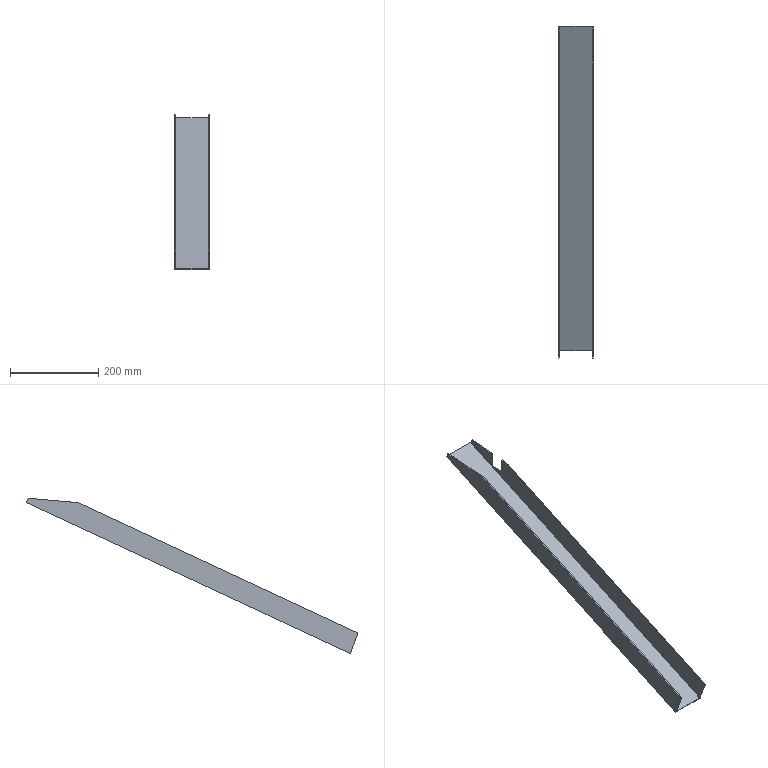Part | NX | features solid 2 | 1 solid | 16 faces | box 78 x 752.166 x 352.381 mm | volume 271303 mm3 | plane 16
STEP:
#1=CARTESIAN_POINT('',(843.,225.865,-160.385));
#2=VERTEX_POINT('',#1);
#3=CARTESIAN_POINT('',(843.,245.,-158.711));
#4=VERTEX_POINT('',#3);
#5=CARTESIAN_POINT('',(843.,-931.001,-261.597));
#6=DIRECTION('',(0.,0.9962,0.08716));
#7=VECTOR('',#6,1000.);
#8=LINE('',#5,#7);
#9=EDGE_CURVE('',#2,#4,#8,.T.);
#10=ORIENTED_EDGE('',*,*,#9,.T.);
#11=CARTESIAN_POINT('',(843.,245.,-190.));
#12=VERTEX_POINT('',#11);
#13=CARTESIAN_POINT('',(843.,245.,-735.668));
#14=DIRECTION('',(0.,0.,-1.));
#15=VECTOR('',#14,1000.);
#16=LINE('',#13,#15);
#17=EDGE_CURVE('',#4,#12,#16,.T.);
#18=ORIENTED_EDGE('',*,*,#17,.T.);
#19=CARTESIAN_POINT('',(843.,275.,-190.));
#20=VERTEX_POINT('',#19);
#21=CARTESIAN_POINT('',(843.,-889.525,-190.));
#22=DIRECTION('',(0.,1.,0.));
#23=VECTOR('',#22,1000.);
#24=LINE('',#21,#23);
#25=EDGE_CURVE('',#12,#20,#24,.T.);
#26=ORIENTED_EDGE('',*,*,#25,.T.);
#27=CARTESIAN_POINT('',(843.,275.,-156.086));
#28=VERTEX_POINT('',#27);
#29=CARTESIAN_POINT('',(843.,275.,-735.668));
#30=DIRECTION('',(0.,0.,-1.));
#31=VECTOR('',#30,1000.);
#32=LINE('',#29,#31);
#33=EDGE_CURVE('',#28,#20,#32,.T.);
#34=ORIENTED_EDGE('',*,*,#33,.F.);
#35=CARTESIAN_POINT('',(843.,340.503,-150.355));
#36=VERTEX_POINT('',#35);
#37=CARTESIAN_POINT('',(843.,-931.001,-261.597));
#38=DIRECTION('',(0.,0.9962,0.08716));
#39=VECTOR('',#38,1000.);
#40=LINE('',#37,#39);
#41=EDGE_CURVE('',#28,#36,#40,.T.);
#42=ORIENTED_EDGE('',*,*,#41,.T.);
#43=CARTESIAN_POINT('',(843.,344.155,-158.187));
#44=VERTEX_POINT('',#43);
#45=CARTESIAN_POINT('',(843.,345.,-160.));
#46=DIRECTION('',(0.,-0.4226,0.9063));
#47=VECTOR('',#46,1000.);
#48=LINE('',#45,#47);
#49=EDGE_CURVE('',#44,#36,#48,.T.);
#50=ORIENTED_EDGE('',*,*,#49,.F.);
#51=CARTESIAN_POINT('',(843.,-390.687,-500.85));
#52=VERTEX_POINT('',#51);
#53=CARTESIAN_POINT('',(843.,-71.454,-351.989));
#54=DIRECTION('',(0.,-0.9063,-0.4226));
#55=VECTOR('',#54,1000.);
#56=LINE('',#53,#55);
#57=EDGE_CURVE('',#44,#52,#56,.T.);
#58=ORIENTED_EDGE('',*,*,#57,.T.);
#59=CARTESIAN_POINT('',(843.,-407.166,-455.572));
#60=VERTEX_POINT('',#59);
#61=CARTESIAN_POINT('',(843.,-373.57,-547.876));
#62=DIRECTION('',(0.,-0.342,0.9397));
#63=VECTOR('',#62,1000.);
#64=LINE('',#61,#63);
#65=EDGE_CURVE('',#52,#60,#64,.T.);
#66=ORIENTED_EDGE('',*,*,#65,.T.);
#67=CARTESIAN_POINT('',(843.,-910.656,-690.353));
#68=DIRECTION('',(0.,-0.9063,-0.4226));
#69=VECTOR('',#68,1000.);
#70=LINE('',#67,#69);
#71=EDGE_CURVE('',#60,#2,#70,.F.);
#72=ORIENTED_EDGE('',*,*,#71,.T.);
#73=EDGE_LOOP('',(#10,#18,#26,#34,#42,#50,#58,#66,#72));
#74=FACE_BOUND('',#73,.T.);
#75=CARTESIAN_POINT('',(843.,-889.525,-735.668));
#76=DIRECTION('',(-1.,0.,0.));
#77=DIRECTION('',(0.,0.08716,-0.9962));
#78=AXIS2_PLACEMENT_3D('',#75,#76,#77);
#79=PLANE('',#78);
#80=ADVANCED_FACE('',(#74),#79,.T.);
#81=CARTESIAN_POINT('',(845.,275.,-190.));
#82=VERTEX_POINT('',#81);
#83=CARTESIAN_POINT('',(845.,245.,-190.));
#84=VERTEX_POINT('',#83);
#85=CARTESIAN_POINT('',(845.,-890.37,-190.));
#86=DIRECTION('',(0.,-1.,0.));
#87=VECTOR('',#86,1000.);
#88=LINE('',#85,#87);
#89=EDGE_CURVE('',#82,#84,#88,.T.);
#90=ORIENTED_EDGE('',*,*,#89,.T.);
#91=CARTESIAN_POINT('',(845.,245.,-158.711));
#92=VERTEX_POINT('',#91);
#93=CARTESIAN_POINT('',(845.,245.,-733.856));
#94=DIRECTION('',(0.,0.,1.));
#95=VECTOR('',#94,1000.);
#96=LINE('',#93,#95);
#97=EDGE_CURVE('',#84,#92,#96,.T.);
#98=ORIENTED_EDGE('',*,*,#97,.T.);
#99=CARTESIAN_POINT('',(845.,225.865,-160.385));
#100=VERTEX_POINT('',#99);
#101=CARTESIAN_POINT('',(845.,-931.682,-261.657));
#102=DIRECTION('',(0.,-0.9962,-0.08716));
#103=VECTOR('',#102,1000.);
#104=LINE('',#101,#103);
#105=EDGE_CURVE('',#92,#100,#104,.T.);
#106=ORIENTED_EDGE('',*,*,#105,.T.);
#107=CARTESIAN_POINT('',(845.,-407.166,-455.572));
#108=VERTEX_POINT('',#107);
#109=CARTESIAN_POINT('',(845.,-910.656,-690.353));
#110=DIRECTION('',(0.,-0.9063,-0.4226));
#111=VECTOR('',#110,1000.);
#112=LINE('',#109,#111);
#113=EDGE_CURVE('',#108,#100,#112,.F.);
#114=ORIENTED_EDGE('',*,*,#113,.F.);
#115=CARTESIAN_POINT('',(845.,-390.,-502.736));
#116=VERTEX_POINT('',#115);
#117=CARTESIAN_POINT('',(845.,-374.252,-546.004));
#118=DIRECTION('',(0.,0.342,-0.9397));
#119=VECTOR('',#118,1000.);
#120=LINE('',#117,#119);
#121=EDGE_CURVE('',#108,#116,#120,.T.);
#122=ORIENTED_EDGE('',*,*,#121,.T.);
#123=CARTESIAN_POINT('',(845.,345.,-160.));
#124=VERTEX_POINT('',#123);
#125=CARTESIAN_POINT('',(845.,-70.609,-353.802));
#126=DIRECTION('',(0.,0.9063,0.4226));
#127=VECTOR('',#126,1000.);
#128=LINE('',#125,#127);
#129=EDGE_CURVE('',#116,#124,#128,.T.);
#130=ORIENTED_EDGE('',*,*,#129,.T.);
#131=CARTESIAN_POINT('',(845.,340.503,-150.355));
#132=VERTEX_POINT('',#131);
#133=CARTESIAN_POINT('',(845.,344.155,-158.187));
#134=DIRECTION('',(0.,0.4226,-0.9063));
#135=VECTOR('',#134,1000.);
#136=LINE('',#133,#135);
#137=EDGE_CURVE('',#132,#124,#136,.T.);
#138=ORIENTED_EDGE('',*,*,#137,.F.);
#139=CARTESIAN_POINT('',(845.,275.,-156.086));
#140=VERTEX_POINT('',#139);
#141=CARTESIAN_POINT('',(845.,-931.682,-261.657));
#142=DIRECTION('',(0.,-0.9962,-0.08716));
#143=VECTOR('',#142,1000.);
#144=LINE('',#141,#143);
#145=EDGE_CURVE('',#132,#140,#144,.T.);
#146=ORIENTED_EDGE('',*,*,#145,.T.);
#147=CARTESIAN_POINT('',(845.,275.,-733.856));
#148=DIRECTION('',(0.,0.,1.));
#149=VECTOR('',#148,1000.);
#150=LINE('',#147,#149);
#151=EDGE_CURVE('',#82,#140,#150,.T.);
#152=ORIENTED_EDGE('',*,*,#151,.F.);
#153=EDGE_LOOP('',(#90,#98,#106,#114,#122,#130,#138,#146,#152));
#154=FACE_BOUND('',#153,.T.);
#155=CARTESIAN_POINT('',(845.,-890.37,-733.856));
#156=DIRECTION('',(1.,0.,0.));
#157=DIRECTION('',(0.,-0.08716,0.9962));
#158=AXIS2_PLACEMENT_3D('',#155,#156,#157);
#159=PLANE('',#158);
#160=ADVANCED_FACE('',(#154),#159,.T.);
#161=CARTESIAN_POINT('',(827.,245.,-158.711));
#162=DIRECTION('',(1.,0.,0.));
#163=VECTOR('',#162,1000.);
#164=LINE('',#161,#163);
#165=EDGE_CURVE('',#4,#92,#164,.T.);
#166=ORIENTED_EDGE('',*,*,#165,.F.);
#167=ORIENTED_EDGE('',*,*,#9,.F.);
#168=CARTESIAN_POINT('',(820.,225.865,-160.385));
#169=DIRECTION('',(1.,0.,0.));
#170=VECTOR('',#169,1000.);
#171=LINE('',#168,#170);
#172=EDGE_CURVE('',#100,#2,#171,.F.);
#173=ORIENTED_EDGE('',*,*,#172,.F.);
#174=ORIENTED_EDGE('',*,*,#105,.F.);
#175=EDGE_LOOP('',(#166,#167,#173,#174));
#176=FACE_BOUND('',#175,.T.);
#177=CARTESIAN_POINT('',(827.,314.243,-152.653));
#178=DIRECTION('',(0.,0.08716,-0.9962));
#179=DIRECTION('',(1.,0.,0.));
#180=AXIS2_PLACEMENT_3D('',#177,#178,#179);
#181=PLANE('',#180);
#182=ADVANCED_FACE('',(#176),#181,.F.);
#183=CARTESIAN_POINT('',(767.,-390.,-502.736));
#184=VERTEX_POINT('',#183);
#185=CARTESIAN_POINT('',(905.,-390.,-502.736));
#186=DIRECTION('',(-1.,0.,0.));
#187=VECTOR('',#186,1000.);
#188=LINE('',#185,#187);
#189=EDGE_CURVE('',#116,#184,#188,.T.);
#190=ORIENTED_EDGE('',*,*,#189,.T.);
#191=CARTESIAN_POINT('',(767.,345.,-160.));
#192=VERTEX_POINT('',#191);
#193=CARTESIAN_POINT('',(767.,-70.609,-353.802));
#194=DIRECTION('',(0.,0.9063,0.4226));
#195=VECTOR('',#194,1000.);
#196=LINE('',#193,#195);
#197=EDGE_CURVE('',#184,#192,#196,.T.);
#198=ORIENTED_EDGE('',*,*,#197,.T.);
#199=CARTESIAN_POINT('',(1300.,345.,-160.));
#200=DIRECTION('',(-1.,0.,0.));
#201=VECTOR('',#200,1000.);
#202=LINE('',#199,#201);
#203=EDGE_CURVE('',#124,#192,#202,.T.);
#204=ORIENTED_EDGE('',*,*,#203,.F.);
#205=ORIENTED_EDGE('',*,*,#129,.F.);
#206=EDGE_LOOP('',(#190,#198,#204,#205));
#207=FACE_BOUND('',#206,.T.);
#208=CARTESIAN_POINT('',(905.,-70.609,-353.802));
#209=DIRECTION('',(0.,0.4226,-0.9063));
#210=DIRECTION('',(0.,0.9063,0.4226));
#211=AXIS2_PLACEMENT_3D('',#208,#209,#210);
#212=PLANE('',#211);
#213=ADVANCED_FACE('',(#207),#212,.T.);
#214=CARTESIAN_POINT('',(769.,-407.166,-455.572));
#215=VERTEX_POINT('',#214);
#216=CARTESIAN_POINT('',(769.,225.865,-160.385));
#217=VERTEX_POINT('',#216);
#218=CARTESIAN_POINT('',(769.,-910.656,-690.353));
#219=DIRECTION('',(0.,0.9063,0.4226));
#220=VECTOR('',#219,1000.);
#221=LINE('',#218,#220);
#222=EDGE_CURVE('',#215,#217,#221,.T.);
#223=ORIENTED_EDGE('',*,*,#222,.T.);
#224=CARTESIAN_POINT('',(767.,225.865,-160.385));
#225=VERTEX_POINT('',#224);
#226=CARTESIAN_POINT('',(750.,225.865,-160.385));
#227=DIRECTION('',(1.,0.,0.));
#228=VECTOR('',#227,1000.);
#229=LINE('',#226,#228);
#230=EDGE_CURVE('',#225,#217,#229,.T.);
#231=ORIENTED_EDGE('',*,*,#230,.F.);
#232=CARTESIAN_POINT('',(767.,-407.166,-455.572));
#233=VERTEX_POINT('',#232);
#234=CARTESIAN_POINT('',(767.,-910.656,-690.353));
#235=DIRECTION('',(0.,0.9063,0.4226));
#236=VECTOR('',#235,1000.);
#237=LINE('',#234,#236);
#238=EDGE_CURVE('',#233,#225,#237,.T.);
#239=ORIENTED_EDGE('',*,*,#238,.F.);
#240=CARTESIAN_POINT('',(750.,-407.166,-455.572));
#241=DIRECTION('',(-1.,0.,0.));
#242=VECTOR('',#241,1000.);
#243=LINE('',#240,#242);
#244=EDGE_CURVE('',#215,#233,#243,.T.);
#245=ORIENTED_EDGE('',*,*,#244,.F.);
#246=EDGE_LOOP('',(#223,#231,#239,#245));
#247=FACE_BOUND('',#246,.T.);
#248=CARTESIAN_POINT('',(750.,-910.656,-690.353));
#249=DIRECTION('',(0.,0.4226,-0.9063));
#250=DIRECTION('',(0.,0.9063,0.4226));
#251=AXIS2_PLACEMENT_3D('',#248,#249,#250);
#252=PLANE('',#251);
#253=ADVANCED_FACE('',(#247),#252,.F.);
#254=CARTESIAN_POINT('',(769.,344.155,-158.187));
#255=VERTEX_POINT('',#254);
#256=CARTESIAN_POINT('',(769.,-390.687,-500.85));
#257=VERTEX_POINT('',#256);
#258=CARTESIAN_POINT('',(769.,-71.454,-351.989));
#259=DIRECTION('',(0.,-0.9063,-0.4226));
#260=VECTOR('',#259,1000.);
#261=LINE('',#258,#260);
#262=EDGE_CURVE('',#255,#257,#261,.T.);
#263=ORIENTED_EDGE('',*,*,#262,.F.);
#264=CARTESIAN_POINT('',(769.,340.503,-150.355));
#265=VERTEX_POINT('',#264);
#266=CARTESIAN_POINT('',(769.,345.,-160.));
#267=DIRECTION('',(0.,-0.4226,0.9063));
#268=VECTOR('',#267,1000.);
#269=LINE('',#266,#268);
#270=EDGE_CURVE('',#255,#265,#269,.T.);
#271=ORIENTED_EDGE('',*,*,#270,.T.);
#272=CARTESIAN_POINT('',(769.,-931.001,-261.597));
#273=DIRECTION('',(0.,0.9962,0.08716));
#274=VECTOR('',#273,1000.);
#275=LINE('',#272,#274);
#276=EDGE_CURVE('',#217,#265,#275,.T.);
#277=ORIENTED_EDGE('',*,*,#276,.F.);
#278=ORIENTED_EDGE('',*,*,#222,.F.);
#279=CARTESIAN_POINT('',(769.,-373.57,-547.876));
#280=DIRECTION('',(0.,-0.342,0.9397));
#281=VECTOR('',#280,1000.);
#282=LINE('',#279,#281);
#283=EDGE_CURVE('',#257,#215,#282,.T.);
#284=ORIENTED_EDGE('',*,*,#283,.F.);
#285=EDGE_LOOP('',(#263,#271,#277,#278,#284));
#286=FACE_BOUND('',#285,.T.);
#287=CARTESIAN_POINT('',(769.,-889.525,-735.668));
#288=DIRECTION('',(-1.,0.,0.));
#289=DIRECTION('',(0.,0.08716,-0.9962));
#290=AXIS2_PLACEMENT_3D('',#287,#288,#289);
#291=PLANE('',#290);
#292=ADVANCED_FACE('',(#286),#291,.F.);
#293=ORIENTED_EDGE('',*,*,#238,.T.);
#294=CARTESIAN_POINT('',(767.,340.503,-150.355));
#295=VERTEX_POINT('',#294);
#296=CARTESIAN_POINT('',(767.,-931.682,-261.657));
#297=DIRECTION('',(0.,-0.9962,-0.08716));
#298=VECTOR('',#297,1000.);
#299=LINE('',#296,#298);
#300=EDGE_CURVE('',#295,#225,#299,.T.);
#301=ORIENTED_EDGE('',*,*,#300,.F.);
#302=CARTESIAN_POINT('',(767.,344.155,-158.187));
#303=DIRECTION('',(0.,0.4226,-0.9063));
#304=VECTOR('',#303,1000.);
#305=LINE('',#302,#304);
#306=EDGE_CURVE('',#295,#192,#305,.T.);
#307=ORIENTED_EDGE('',*,*,#306,.T.);
#308=ORIENTED_EDGE('',*,*,#197,.F.);
#309=CARTESIAN_POINT('',(767.,-374.252,-546.004));
#310=DIRECTION('',(0.,0.342,-0.9397));
#311=VECTOR('',#310,1000.);
#312=LINE('',#309,#311);
#313=EDGE_CURVE('',#233,#184,#312,.T.);
#314=ORIENTED_EDGE('',*,*,#313,.F.);
#315=EDGE_LOOP('',(#293,#301,#307,#308,#314));
#316=FACE_BOUND('',#315,.T.);
#317=CARTESIAN_POINT('',(767.,-890.37,-733.856));
#318=DIRECTION('',(1.,0.,0.));
#319=DIRECTION('',(0.,-0.08716,0.9962));
#320=AXIS2_PLACEMENT_3D('',#317,#318,#319);
#321=PLANE('',#320);
#322=ADVANCED_FACE('',(#316),#321,.F.);
#323=CARTESIAN_POINT('',(820.,-407.166,-455.572));
#324=DIRECTION('',(-1.,0.,0.));
#325=VECTOR('',#324,1000.);
#326=LINE('',#323,#325);
#327=EDGE_CURVE('',#60,#108,#326,.F.);
#328=ORIENTED_EDGE('',*,*,#327,.T.);
#329=ORIENTED_EDGE('',*,*,#113,.T.);
#330=ORIENTED_EDGE('',*,*,#172,.T.);
#331=ORIENTED_EDGE('',*,*,#71,.F.);
#332=EDGE_LOOP('',(#328,#329,#330,#331));
#333=FACE_BOUND('',#332,.T.);
#334=CARTESIAN_POINT('',(820.,-910.656,-690.353));
#335=DIRECTION('',(0.,0.4226,-0.9063));
#336=DIRECTION('',(0.,0.9063,0.4226));
#337=AXIS2_PLACEMENT_3D('',#334,#335,#336);
#338=PLANE('',#337);
#339=ADVANCED_FACE('',(#333),#338,.F.);
#340=ORIENTED_EDGE('',*,*,#57,.F.);
#341=CARTESIAN_POINT('',(1300.,344.155,-158.187));
#342=DIRECTION('',(-1.,0.,0.));
#343=VECTOR('',#342,1000.);
#344=LINE('',#341,#343);
#345=EDGE_CURVE('',#44,#255,#344,.T.);
#346=ORIENTED_EDGE('',*,*,#345,.T.);
#347=ORIENTED_EDGE('',*,*,#262,.T.);
#348=CARTESIAN_POINT('',(905.,-390.687,-500.85));
#349=DIRECTION('',(-1.,0.,0.));
#350=VECTOR('',#349,1000.);
#351=LINE('',#348,#350);
#352=EDGE_CURVE('',#52,#257,#351,.T.);
#353=ORIENTED_EDGE('',*,*,#352,.F.);
#354=EDGE_LOOP('',(#340,#346,#347,#353));
#355=FACE_BOUND('',#354,.T.);
#356=CARTESIAN_POINT('',(905.,-71.454,-351.989));
#357=DIRECTION('',(0.,0.4226,-0.9063));
#358=DIRECTION('',(0.,0.9063,0.4226));
#359=AXIS2_PLACEMENT_3D('',#356,#357,#358);
#360=PLANE('',#359);
#361=ADVANCED_FACE('',(#355),#360,.F.);
#362=CARTESIAN_POINT('',(1300.,340.503,-150.355));
#363=DIRECTION('',(1.,0.,0.));
#364=VECTOR('',#363,1000.);
#365=LINE('',#362,#364);
#366=EDGE_CURVE('',#295,#265,#365,.T.);
#367=ORIENTED_EDGE('',*,*,#366,.T.);
#368=ORIENTED_EDGE('',*,*,#270,.F.);
#369=ORIENTED_EDGE('',*,*,#345,.F.);
#370=ORIENTED_EDGE('',*,*,#49,.T.);
#371=CARTESIAN_POINT('',(1300.,340.503,-150.355));
#372=DIRECTION('',(1.,0.,0.));
#373=VECTOR('',#372,1000.);
#374=LINE('',#371,#373);
#375=EDGE_CURVE('',#36,#132,#374,.T.);
#376=ORIENTED_EDGE('',*,*,#375,.T.);
#377=ORIENTED_EDGE('',*,*,#137,.T.);
#378=ORIENTED_EDGE('',*,*,#203,.T.);
#379=ORIENTED_EDGE('',*,*,#306,.F.);
#380=EDGE_LOOP('',(#367,#368,#369,#370,#376,#377,#378,#379));
#381=FACE_BOUND('',#380,.T.);
#382=CARTESIAN_POINT('',(1300.,344.155,-158.187));
#383=DIRECTION('',(0.,0.9063,0.4226));
#384=DIRECTION('',(0.,-0.4226,0.9063));
#385=AXIS2_PLACEMENT_3D('',#382,#383,#384);
#386=PLANE('',#385);
#387=ADVANCED_FACE('',(#381),#386,.T.);
#388=ORIENTED_EDGE('',*,*,#41,.F.);
#389=CARTESIAN_POINT('',(827.,275.,-156.086));
#390=DIRECTION('',(1.,0.,0.));
#391=VECTOR('',#390,1000.);
#392=LINE('',#389,#391);
#393=EDGE_CURVE('',#28,#140,#392,.T.);
#394=ORIENTED_EDGE('',*,*,#393,.T.);
#395=ORIENTED_EDGE('',*,*,#145,.F.);
#396=ORIENTED_EDGE('',*,*,#375,.F.);
#397=EDGE_LOOP('',(#388,#394,#395,#396));
#398=FACE_BOUND('',#397,.T.);
#399=CARTESIAN_POINT('',(827.,314.243,-152.653));
#400=DIRECTION('',(0.,0.08716,-0.9962));
#401=DIRECTION('',(1.,0.,0.));
#402=AXIS2_PLACEMENT_3D('',#399,#400,#401);
#403=PLANE('',#402);
#404=ADVANCED_FACE('',(#398),#403,.F.);
#405=ORIENTED_EDGE('',*,*,#300,.T.);
#406=ORIENTED_EDGE('',*,*,#230,.T.);
#407=ORIENTED_EDGE('',*,*,#276,.T.);
#408=ORIENTED_EDGE('',*,*,#366,.F.);
#409=EDGE_LOOP('',(#405,#406,#407,#408));
#410=FACE_BOUND('',#409,.T.);
#411=CARTESIAN_POINT('',(827.,314.243,-152.653));
#412=DIRECTION('',(0.,0.08716,-0.9962));
#413=DIRECTION('',(1.,0.,0.));
#414=AXIS2_PLACEMENT_3D('',#411,#412,#413);
#415=PLANE('',#414);
#416=ADVANCED_FACE('',(#410),#415,.F.);
#417=ORIENTED_EDGE('',*,*,#121,.F.);
#418=ORIENTED_EDGE('',*,*,#327,.F.);
#419=ORIENTED_EDGE('',*,*,#65,.F.);
#420=ORIENTED_EDGE('',*,*,#352,.T.);
#421=ORIENTED_EDGE('',*,*,#283,.T.);
#422=ORIENTED_EDGE('',*,*,#244,.T.);
#423=ORIENTED_EDGE('',*,*,#313,.T.);
#424=ORIENTED_EDGE('',*,*,#189,.F.);
#425=EDGE_LOOP('',(#417,#418,#419,#420,#421,#422,#423,#424));
#426=FACE_BOUND('',#425,.T.);
#427=CARTESIAN_POINT('',(825.,-390.,-502.736));
#428=DIRECTION('',(0.,0.9397,0.342));
#429=DIRECTION('',(0.,-0.342,0.9397));
#430=AXIS2_PLACEMENT_3D('',#427,#428,#429);
#431=PLANE('',#430);
#432=ADVANCED_FACE('',(#426),#431,.F.);
#433=ORIENTED_EDGE('',*,*,#165,.T.);
#434=ORIENTED_EDGE('',*,*,#97,.F.);
#435=CARTESIAN_POINT('',(0.,245.,-190.));
#436=DIRECTION('',(1.,0.,0.));
#437=VECTOR('',#436,1000.);
#438=LINE('',#435,#437);
#439=EDGE_CURVE('',#12,#84,#438,.T.);
#440=ORIENTED_EDGE('',*,*,#439,.F.);
#441=ORIENTED_EDGE('',*,*,#17,.F.);
#442=EDGE_LOOP('',(#433,#434,#440,#441));
#443=FACE_BOUND('',#442,.T.);
#444=CARTESIAN_POINT('',(0.,245.,-90.));
#445=DIRECTION('',(0.,1.,0.));
#446=DIRECTION('',(0.,0.,1.));
#447=AXIS2_PLACEMENT_3D('',#444,#445,#446);
#448=PLANE('',#447);
#449=ADVANCED_FACE('',(#443),#448,.T.);
#450=ORIENTED_EDGE('',*,*,#33,.T.);
#451=CARTESIAN_POINT('',(0.,275.,-190.));
#452=DIRECTION('',(1.,0.,0.));
#453=VECTOR('',#452,1000.);
#454=LINE('',#451,#453);
#455=EDGE_CURVE('',#20,#82,#454,.T.);
#456=ORIENTED_EDGE('',*,*,#455,.T.);
#457=ORIENTED_EDGE('',*,*,#151,.T.);
#458=ORIENTED_EDGE('',*,*,#393,.F.);
#459=EDGE_LOOP('',(#450,#456,#457,#458));
#460=FACE_BOUND('',#459,.T.);
#461=CARTESIAN_POINT('',(0.,275.,-90.));
#462=DIRECTION('',(0.,1.,0.));
#463=DIRECTION('',(0.,0.,1.));
#464=AXIS2_PLACEMENT_3D('',#461,#462,#463);
#465=PLANE('',#464);
#466=ADVANCED_FACE('',(#460),#465,.F.);
#467=ORIENTED_EDGE('',*,*,#439,.T.);
#468=ORIENTED_EDGE('',*,*,#89,.F.);
#469=ORIENTED_EDGE('',*,*,#455,.F.);
#470=ORIENTED_EDGE('',*,*,#25,.F.);
#471=EDGE_LOOP('',(#467,#468,#469,#470));
#472=FACE_BOUND('',#471,.T.);
#473=CARTESIAN_POINT('',(422.5,130.,-190.));
#474=DIRECTION('',(0.,0.,1.));
#475=DIRECTION('',(1.,0.,0.));
#476=AXIS2_PLACEMENT_3D('',#473,#474,#475);
#477=PLANE('',#476);
#478=ADVANCED_FACE('',(#472),#477,.T.);
#479=CLOSED_SHELL('',(#80,#160,#182,#213,#253,#292,#322,#339,#361,#387,#404,#416,#432,#449,#466,#478));
#480=MANIFOLD_SOLID_BREP('',#479);
#481=(LENGTH_UNIT()NAMED_UNIT(*)SI_UNIT(.MILLI.,.METRE.));
#482=UNCERTAINTY_MEASURE_WITH_UNIT(LENGTH_MEASURE(0.00001),#481,'','');
#483=(NAMED_UNIT(*)PLANE_ANGLE_UNIT()SI_UNIT($,.RADIAN.));
#484=(NAMED_UNIT(*)SI_UNIT($,.STERADIAN.)SOLID_ANGLE_UNIT());
#485=(GEOMETRIC_REPRESENTATION_CONTEXT(3)GLOBAL_UNCERTAINTY_ASSIGNED_CONTEXT((#482))GLOBAL_UNIT_ASSIGNED_CONTEXT((#481,#483,#484))REPRESENTATION_CONTEXT('',''));
#486=ADVANCED_BREP_SHAPE_REPRESENTATION('',(#480),#485);